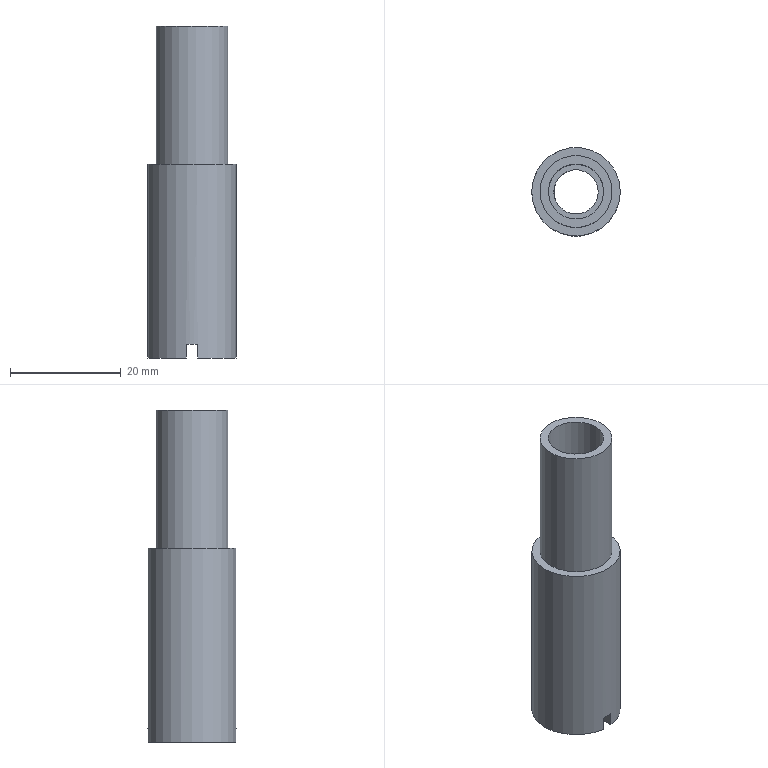Part | NX | features solid 2 | 1 solid | 15 faces | box 16 x 16 x 60 mm | volume 5886 mm3 | plane 11 | cylinder 4 | commonest cylinder face diameters 8 x1 10 x1 13 x1 16 x1
STEP:
#1=CARTESIAN_POINT('',(-774.,-102.937,70.5));
#2=VERTEX_POINT('',#1);
#3=CARTESIAN_POINT('',(-774.,-102.937,68.));
#4=VERTEX_POINT('',#3);
#5=CARTESIAN_POINT('',(-774.,-102.937,128.));
#6=DIRECTION('',(0.,0.,-1.));
#7=VECTOR('',#6,1000.);
#8=LINE('',#5,#7);
#9=EDGE_CURVE('',#2,#4,#8,.T.);
#10=ORIENTED_EDGE('',*,*,#9,.T.);
#11=CARTESIAN_POINT('',(-774.,-87.063,68.));
#12=VERTEX_POINT('',#11);
#13=CARTESIAN_POINT('',(-775.,-95.,68.));
#14=DIRECTION('',(0.,0.,1.));
#15=DIRECTION('',(1.,0.,0.));
#16=AXIS2_PLACEMENT_3D('',#13,#14,#15);
#17=CIRCLE('',#16,8.);
#18=EDGE_CURVE('',#4,#12,#17,.T.);
#19=ORIENTED_EDGE('',*,*,#18,.T.);
#20=CARTESIAN_POINT('',(-774.,-87.063,70.5));
#21=VERTEX_POINT('',#20);
#22=CARTESIAN_POINT('',(-774.,-87.063,128.));
#23=DIRECTION('',(0.,0.,-1.));
#24=VECTOR('',#23,1000.);
#25=LINE('',#22,#24);
#26=EDGE_CURVE('',#12,#21,#25,.F.);
#27=ORIENTED_EDGE('',*,*,#26,.T.);
#28=CARTESIAN_POINT('',(-776.,-87.063,70.5));
#29=VERTEX_POINT('',#28);
#30=CARTESIAN_POINT('',(-775.,-95.,70.5));
#31=DIRECTION('',(0.,0.,1.));
#32=DIRECTION('',(1.,0.,0.));
#33=AXIS2_PLACEMENT_3D('',#30,#31,#32);
#34=CIRCLE('',#33,8.);
#35=EDGE_CURVE('',#21,#29,#34,.T.);
#36=ORIENTED_EDGE('',*,*,#35,.T.);
#37=CARTESIAN_POINT('',(-776.,-87.063,68.));
#38=VERTEX_POINT('',#37);
#39=CARTESIAN_POINT('',(-776.,-87.063,128.));
#40=DIRECTION('',(0.,0.,-1.));
#41=VECTOR('',#40,1000.);
#42=LINE('',#39,#41);
#43=EDGE_CURVE('',#38,#29,#42,.F.);
#44=ORIENTED_EDGE('',*,*,#43,.F.);
#45=CARTESIAN_POINT('',(-776.,-102.937,68.));
#46=VERTEX_POINT('',#45);
#47=CARTESIAN_POINT('',(-775.,-95.,68.));
#48=DIRECTION('',(0.,0.,1.));
#49=DIRECTION('',(1.,0.,0.));
#50=AXIS2_PLACEMENT_3D('',#47,#48,#49);
#51=CIRCLE('',#50,8.);
#52=EDGE_CURVE('',#38,#46,#51,.T.);
#53=ORIENTED_EDGE('',*,*,#52,.T.);
#54=CARTESIAN_POINT('',(-776.,-102.937,70.5));
#55=VERTEX_POINT('',#54);
#56=CARTESIAN_POINT('',(-776.,-102.937,128.));
#57=DIRECTION('',(0.,0.,-1.));
#58=VECTOR('',#57,1000.);
#59=LINE('',#56,#58);
#60=EDGE_CURVE('',#55,#46,#59,.T.);
#61=ORIENTED_EDGE('',*,*,#60,.F.);
#62=CARTESIAN_POINT('',(-775.,-95.,70.5));
#63=DIRECTION('',(0.,0.,1.));
#64=DIRECTION('',(1.,0.,0.));
#65=AXIS2_PLACEMENT_3D('',#62,#63,#64);
#66=CIRCLE('',#65,8.);
#67=EDGE_CURVE('',#55,#2,#66,.T.);
#68=ORIENTED_EDGE('',*,*,#67,.T.);
#69=EDGE_LOOP('',(#10,#19,#27,#36,#44,#53,#61,#68));
#70=FACE_BOUND('',#69,.T.);
#71=CARTESIAN_POINT('',(-783.,-95.,103.));
#72=VERTEX_POINT('',#71);
#73=CARTESIAN_POINT('',(-775.,-95.,103.));
#74=DIRECTION('',(0.,0.,-1.));
#75=DIRECTION('',(-1.,0.,0.));
#76=AXIS2_PLACEMENT_3D('',#73,#74,#75);
#77=CIRCLE('',#76,8.);
#78=EDGE_CURVE('',#72,#72,#77,.F.);
#79=ORIENTED_EDGE('',*,*,#78,.F.);
#80=EDGE_LOOP('',(#79));
#81=FACE_BOUND('',#80,.T.);
#82=CARTESIAN_POINT('',(-775.,-95.,128.));
#83=DIRECTION('',(0.,0.,-1.));
#84=DIRECTION('',(1.,0.,0.));
#85=AXIS2_PLACEMENT_3D('',#82,#83,#84);
#86=CYLINDRICAL_SURFACE('',#85,8.);
#87=ADVANCED_FACE('',(#70,#81),#86,.T.);
#88=ORIENTED_EDGE('',*,*,#52,.F.);
#89=CARTESIAN_POINT('',(-776.,-91.127,68.));
#90=VERTEX_POINT('',#89);
#91=CARTESIAN_POINT('',(-776.,-87.,68.));
#92=DIRECTION('',(0.,1.,0.));
#93=VECTOR('',#92,1000.);
#94=LINE('',#91,#93);
#95=EDGE_CURVE('',#38,#90,#94,.F.);
#96=ORIENTED_EDGE('',*,*,#95,.T.);
#97=CARTESIAN_POINT('',(-776.,-98.873,68.));
#98=VERTEX_POINT('',#97);
#99=CARTESIAN_POINT('',(-775.,-95.,68.));
#100=DIRECTION('',(0.,0.,1.));
#101=DIRECTION('',(1.,0.,0.));
#102=AXIS2_PLACEMENT_3D('',#99,#100,#101);
#103=CIRCLE('',#102,4.);
#104=EDGE_CURVE('',#90,#98,#103,.T.);
#105=ORIENTED_EDGE('',*,*,#104,.T.);
#106=CARTESIAN_POINT('',(-776.,-87.,68.));
#107=DIRECTION('',(0.,1.,0.));
#108=VECTOR('',#107,1000.);
#109=LINE('',#106,#108);
#110=EDGE_CURVE('',#98,#46,#109,.F.);
#111=ORIENTED_EDGE('',*,*,#110,.T.);
#112=EDGE_LOOP('',(#88,#96,#105,#111));
#113=FACE_BOUND('',#112,.T.);
#114=CARTESIAN_POINT('',(-775.,-95.,68.));
#115=DIRECTION('',(0.,0.,-1.));
#116=DIRECTION('',(1.,0.,0.));
#117=AXIS2_PLACEMENT_3D('',#114,#115,#116);
#118=PLANE('',#117);
#119=ADVANCED_FACE('',(#113),#118,.T.);
#120=CARTESIAN_POINT('',(-774.,-98.873,68.));
#121=VERTEX_POINT('',#120);
#122=CARTESIAN_POINT('',(-774.,-87.,68.));
#123=DIRECTION('',(0.,1.,0.));
#124=VECTOR('',#123,1000.);
#125=LINE('',#122,#124);
#126=EDGE_CURVE('',#121,#4,#125,.F.);
#127=ORIENTED_EDGE('',*,*,#126,.F.);
#128=CARTESIAN_POINT('',(-774.,-91.127,68.));
#129=VERTEX_POINT('',#128);
#130=CARTESIAN_POINT('',(-775.,-95.,68.));
#131=DIRECTION('',(0.,0.,1.));
#132=DIRECTION('',(1.,0.,0.));
#133=AXIS2_PLACEMENT_3D('',#130,#131,#132);
#134=CIRCLE('',#133,4.);
#135=EDGE_CURVE('',#121,#129,#134,.T.);
#136=ORIENTED_EDGE('',*,*,#135,.T.);
#137=CARTESIAN_POINT('',(-774.,-87.,68.));
#138=DIRECTION('',(0.,1.,0.));
#139=VECTOR('',#138,1000.);
#140=LINE('',#137,#139);
#141=EDGE_CURVE('',#12,#129,#140,.F.);
#142=ORIENTED_EDGE('',*,*,#141,.F.);
#143=ORIENTED_EDGE('',*,*,#18,.F.);
#144=EDGE_LOOP('',(#127,#136,#142,#143));
#145=FACE_BOUND('',#144,.T.);
#146=CARTESIAN_POINT('',(-775.,-95.,68.));
#147=DIRECTION('',(0.,0.,-1.));
#148=DIRECTION('',(1.,0.,0.));
#149=AXIS2_PLACEMENT_3D('',#146,#147,#148);
#150=PLANE('',#149);
#151=ADVANCED_FACE('',(#145),#150,.T.);
#152=ORIENTED_EDGE('',*,*,#78,.T.);
#153=EDGE_LOOP('',(#152));
#154=FACE_BOUND('',#153,.T.);
#155=CARTESIAN_POINT('',(-768.5,-95.,103.));
#156=VERTEX_POINT('',#155);
#157=CARTESIAN_POINT('',(-775.,-95.,103.));
#158=DIRECTION('',(0.,0.,1.));
#159=DIRECTION('',(1.,0.,0.));
#160=AXIS2_PLACEMENT_3D('',#157,#158,#159);
#161=CIRCLE('',#160,6.5);
#162=EDGE_CURVE('',#156,#156,#161,.T.);
#163=ORIENTED_EDGE('',*,*,#162,.F.);
#164=EDGE_LOOP('',(#163));
#165=FACE_BOUND('',#164,.T.);
#166=CARTESIAN_POINT('',(-775.,-95.,103.));
#167=DIRECTION('',(0.,0.,1.));
#168=DIRECTION('',(-1.,0.,0.));
#169=AXIS2_PLACEMENT_3D('',#166,#167,#168);
#170=PLANE('',#169);
#171=ADVANCED_FACE('',(#154,#165),#170,.T.);
#172=CARTESIAN_POINT('',(-768.5,-95.,128.));
#173=VERTEX_POINT('',#172);
#174=CARTESIAN_POINT('',(-775.,-95.,128.));
#175=DIRECTION('',(0.,0.,1.));
#176=DIRECTION('',(1.,0.,0.));
#177=AXIS2_PLACEMENT_3D('',#174,#175,#176);
#178=CIRCLE('',#177,6.5);
#179=EDGE_CURVE('',#173,#173,#178,.T.);
#180=ORIENTED_EDGE('',*,*,#179,.F.);
#181=EDGE_LOOP('',(#180));
#182=FACE_BOUND('',#181,.T.);
#183=ORIENTED_EDGE('',*,*,#162,.T.);
#184=EDGE_LOOP('',(#183));
#185=FACE_BOUND('',#184,.T.);
#186=CARTESIAN_POINT('',(-775.,-95.,103.));
#187=DIRECTION('',(0.,0.,1.));
#188=DIRECTION('',(-1.,0.,0.));
#189=AXIS2_PLACEMENT_3D('',#186,#187,#188);
#190=CYLINDRICAL_SURFACE('',#189,6.5);
#191=ADVANCED_FACE('',(#182,#185),#190,.T.);
#192=CARTESIAN_POINT('',(-770.,-95.,128.));
#193=VERTEX_POINT('',#192);
#194=CARTESIAN_POINT('',(-775.,-95.,128.));
#195=DIRECTION('',(0.,0.,1.));
#196=DIRECTION('',(1.,0.,0.));
#197=AXIS2_PLACEMENT_3D('',#194,#195,#196);
#198=CIRCLE('',#197,5.);
#199=EDGE_CURVE('',#193,#193,#198,.T.);
#200=ORIENTED_EDGE('',*,*,#199,.F.);
#201=EDGE_LOOP('',(#200));
#202=FACE_BOUND('',#201,.T.);
#203=ORIENTED_EDGE('',*,*,#179,.T.);
#204=EDGE_LOOP('',(#203));
#205=FACE_BOUND('',#204,.T.);
#206=CARTESIAN_POINT('',(-775.,-95.,128.));
#207=DIRECTION('',(0.,0.,-1.));
#208=DIRECTION('',(1.,0.,0.));
#209=AXIS2_PLACEMENT_3D('',#206,#207,#208);
#210=PLANE('',#209);
#211=ADVANCED_FACE('',(#202,#205),#210,.F.);
#212=CARTESIAN_POINT('',(-771.,-95.,78.));
#213=VERTEX_POINT('',#212);
#214=CARTESIAN_POINT('',(-775.,-95.,78.));
#215=DIRECTION('',(0.,0.,1.));
#216=DIRECTION('',(1.,0.,0.));
#217=AXIS2_PLACEMENT_3D('',#214,#215,#216);
#218=CIRCLE('',#217,4.);
#219=EDGE_CURVE('',#213,#213,#218,.F.);
#220=ORIENTED_EDGE('',*,*,#219,.F.);
#221=EDGE_LOOP('',(#220));
#222=FACE_BOUND('',#221,.T.);
#223=ORIENTED_EDGE('',*,*,#135,.F.);
#224=CARTESIAN_POINT('',(-774.,-98.873,70.5));
#225=VERTEX_POINT('',#224);
#226=CARTESIAN_POINT('',(-774.,-98.873,78.));
#227=DIRECTION('',(0.,0.,-1.));
#228=VECTOR('',#227,1000.);
#229=LINE('',#226,#228);
#230=EDGE_CURVE('',#225,#121,#229,.T.);
#231=ORIENTED_EDGE('',*,*,#230,.F.);
#232=CARTESIAN_POINT('',(-776.,-98.873,70.5));
#233=VERTEX_POINT('',#232);
#234=CARTESIAN_POINT('',(-775.,-95.,70.5));
#235=DIRECTION('',(0.,0.,1.));
#236=DIRECTION('',(1.,0.,0.));
#237=AXIS2_PLACEMENT_3D('',#234,#235,#236);
#238=CIRCLE('',#237,4.);
#239=EDGE_CURVE('',#233,#225,#238,.T.);
#240=ORIENTED_EDGE('',*,*,#239,.F.);
#241=CARTESIAN_POINT('',(-776.,-98.873,78.));
#242=DIRECTION('',(0.,0.,-1.));
#243=VECTOR('',#242,1000.);
#244=LINE('',#241,#243);
#245=EDGE_CURVE('',#233,#98,#244,.T.);
#246=ORIENTED_EDGE('',*,*,#245,.T.);
#247=ORIENTED_EDGE('',*,*,#104,.F.);
#248=CARTESIAN_POINT('',(-776.,-91.127,70.5));
#249=VERTEX_POINT('',#248);
#250=CARTESIAN_POINT('',(-776.,-91.127,78.));
#251=DIRECTION('',(0.,0.,-1.));
#252=VECTOR('',#251,1000.);
#253=LINE('',#250,#252);
#254=EDGE_CURVE('',#90,#249,#253,.F.);
#255=ORIENTED_EDGE('',*,*,#254,.T.);
#256=CARTESIAN_POINT('',(-774.,-91.127,70.5));
#257=VERTEX_POINT('',#256);
#258=CARTESIAN_POINT('',(-775.,-95.,70.5));
#259=DIRECTION('',(0.,0.,1.));
#260=DIRECTION('',(1.,0.,0.));
#261=AXIS2_PLACEMENT_3D('',#258,#259,#260);
#262=CIRCLE('',#261,4.);
#263=EDGE_CURVE('',#257,#249,#262,.T.);
#264=ORIENTED_EDGE('',*,*,#263,.F.);
#265=CARTESIAN_POINT('',(-774.,-91.127,78.));
#266=DIRECTION('',(0.,0.,-1.));
#267=VECTOR('',#266,1000.);
#268=LINE('',#265,#267);
#269=EDGE_CURVE('',#129,#257,#268,.F.);
#270=ORIENTED_EDGE('',*,*,#269,.F.);
#271=EDGE_LOOP('',(#223,#231,#240,#246,#247,#255,#264,#270));
#272=FACE_BOUND('',#271,.T.);
#273=CARTESIAN_POINT('',(-775.,-95.,78.));
#274=DIRECTION('',(0.,0.,-1.));
#275=DIRECTION('',(1.,0.,0.));
#276=AXIS2_PLACEMENT_3D('',#273,#274,#275);
#277=CYLINDRICAL_SURFACE('',#276,4.);
#278=ADVANCED_FACE('',(#222,#272),#277,.F.);
#279=CARTESIAN_POINT('',(-770.,-95.,78.));
#280=VERTEX_POINT('',#279);
#281=CARTESIAN_POINT('',(-775.,-95.,78.));
#282=DIRECTION('',(0.,0.,1.));
#283=DIRECTION('',(1.,0.,0.));
#284=AXIS2_PLACEMENT_3D('',#281,#282,#283);
#285=CIRCLE('',#284,5.);
#286=EDGE_CURVE('',#280,#280,#285,.T.);
#287=ORIENTED_EDGE('',*,*,#286,.T.);
#288=EDGE_LOOP('',(#287));
#289=FACE_BOUND('',#288,.T.);
#290=ORIENTED_EDGE('',*,*,#219,.T.);
#291=EDGE_LOOP('',(#290));
#292=FACE_BOUND('',#291,.T.);
#293=CARTESIAN_POINT('',(-775.,-95.,78.));
#294=DIRECTION('',(0.,0.,-1.));
#295=DIRECTION('',(1.,0.,0.));
#296=AXIS2_PLACEMENT_3D('',#293,#294,#295);
#297=PLANE('',#296);
#298=ADVANCED_FACE('',(#289,#292),#297,.F.);
#299=ORIENTED_EDGE('',*,*,#199,.T.);
#300=EDGE_LOOP('',(#299));
#301=FACE_BOUND('',#300,.T.);
#302=ORIENTED_EDGE('',*,*,#286,.F.);
#303=EDGE_LOOP('',(#302));
#304=FACE_BOUND('',#303,.T.);
#305=CARTESIAN_POINT('',(-775.,-95.,128.));
#306=DIRECTION('',(0.,0.,-1.));
#307=DIRECTION('',(1.,0.,0.));
#308=AXIS2_PLACEMENT_3D('',#305,#306,#307);
#309=CYLINDRICAL_SURFACE('',#308,5.);
#310=ADVANCED_FACE('',(#301,#304),#309,.F.);
#311=ORIENTED_EDGE('',*,*,#9,.F.);
#312=CARTESIAN_POINT('',(-774.,-87.,70.5));
#313=DIRECTION('',(0.,1.,0.));
#314=VECTOR('',#313,1000.);
#315=LINE('',#312,#314);
#316=EDGE_CURVE('',#225,#2,#315,.F.);
#317=ORIENTED_EDGE('',*,*,#316,.F.);
#318=ORIENTED_EDGE('',*,*,#230,.T.);
#319=ORIENTED_EDGE('',*,*,#126,.T.);
#320=EDGE_LOOP('',(#311,#317,#318,#319));
#321=FACE_BOUND('',#320,.T.);
#322=CARTESIAN_POINT('',(-774.,-87.,68.));
#323=DIRECTION('',(1.,0.,0.));
#324=DIRECTION('',(0.,0.,1.));
#325=AXIS2_PLACEMENT_3D('',#322,#323,#324);
#326=PLANE('',#325);
#327=ADVANCED_FACE('',(#321),#326,.F.);
#328=CARTESIAN_POINT('',(-776.,-87.,70.5));
#329=DIRECTION('',(0.,1.,0.));
#330=VECTOR('',#329,1000.);
#331=LINE('',#328,#330);
#332=EDGE_CURVE('',#233,#55,#331,.F.);
#333=ORIENTED_EDGE('',*,*,#332,.T.);
#334=ORIENTED_EDGE('',*,*,#60,.T.);
#335=ORIENTED_EDGE('',*,*,#110,.F.);
#336=ORIENTED_EDGE('',*,*,#245,.F.);
#337=EDGE_LOOP('',(#333,#334,#335,#336));
#338=FACE_BOUND('',#337,.T.);
#339=CARTESIAN_POINT('',(-776.,-87.,68.));
#340=DIRECTION('',(1.,0.,0.));
#341=DIRECTION('',(0.,0.,1.));
#342=AXIS2_PLACEMENT_3D('',#339,#340,#341);
#343=PLANE('',#342);
#344=ADVANCED_FACE('',(#338),#343,.T.);
#345=ORIENTED_EDGE('',*,*,#67,.F.);
#346=ORIENTED_EDGE('',*,*,#332,.F.);
#347=ORIENTED_EDGE('',*,*,#239,.T.);
#348=ORIENTED_EDGE('',*,*,#316,.T.);
#349=EDGE_LOOP('',(#345,#346,#347,#348));
#350=FACE_BOUND('',#349,.T.);
#351=CARTESIAN_POINT('',(-775.,-87.,70.5));
#352=DIRECTION('',(0.,0.,-1.));
#353=DIRECTION('',(0.,-1.,0.));
#354=AXIS2_PLACEMENT_3D('',#351,#352,#353);
#355=PLANE('',#354);
#356=ADVANCED_FACE('',(#350),#355,.T.);
#357=ORIENTED_EDGE('',*,*,#35,.F.);
#358=CARTESIAN_POINT('',(-774.,-87.,70.5));
#359=DIRECTION('',(0.,1.,0.));
#360=VECTOR('',#359,1000.);
#361=LINE('',#358,#360);
#362=EDGE_CURVE('',#21,#257,#361,.F.);
#363=ORIENTED_EDGE('',*,*,#362,.T.);
#364=ORIENTED_EDGE('',*,*,#263,.T.);
#365=CARTESIAN_POINT('',(-776.,-87.,70.5));
#366=DIRECTION('',(0.,1.,0.));
#367=VECTOR('',#366,1000.);
#368=LINE('',#365,#367);
#369=EDGE_CURVE('',#29,#249,#368,.F.);
#370=ORIENTED_EDGE('',*,*,#369,.F.);
#371=EDGE_LOOP('',(#357,#363,#364,#370));
#372=FACE_BOUND('',#371,.T.);
#373=CARTESIAN_POINT('',(-775.,-87.,70.5));
#374=DIRECTION('',(0.,0.,-1.));
#375=DIRECTION('',(0.,-1.,0.));
#376=AXIS2_PLACEMENT_3D('',#373,#374,#375);
#377=PLANE('',#376);
#378=ADVANCED_FACE('',(#372),#377,.T.);
#379=ORIENTED_EDGE('',*,*,#26,.F.);
#380=ORIENTED_EDGE('',*,*,#141,.T.);
#381=ORIENTED_EDGE('',*,*,#269,.T.);
#382=ORIENTED_EDGE('',*,*,#362,.F.);
#383=EDGE_LOOP('',(#379,#380,#381,#382));
#384=FACE_BOUND('',#383,.T.);
#385=CARTESIAN_POINT('',(-774.,-87.,68.));
#386=DIRECTION('',(1.,0.,0.));
#387=DIRECTION('',(0.,0.,1.));
#388=AXIS2_PLACEMENT_3D('',#385,#386,#387);
#389=PLANE('',#388);
#390=ADVANCED_FACE('',(#384),#389,.F.);
#391=ORIENTED_EDGE('',*,*,#95,.F.);
#392=ORIENTED_EDGE('',*,*,#43,.T.);
#393=ORIENTED_EDGE('',*,*,#369,.T.);
#394=ORIENTED_EDGE('',*,*,#254,.F.);
#395=EDGE_LOOP('',(#391,#392,#393,#394));
#396=FACE_BOUND('',#395,.T.);
#397=CARTESIAN_POINT('',(-776.,-87.,68.));
#398=DIRECTION('',(1.,0.,0.));
#399=DIRECTION('',(0.,0.,1.));
#400=AXIS2_PLACEMENT_3D('',#397,#398,#399);
#401=PLANE('',#400);
#402=ADVANCED_FACE('',(#396),#401,.T.);
#403=CLOSED_SHELL('',(#87,#119,#151,#171,#191,#211,#278,#298,#310,#327,#344,#356,#378,#390,#402));
#404=MANIFOLD_SOLID_BREP('',#403);
#405=(LENGTH_UNIT()NAMED_UNIT(*)SI_UNIT(.MILLI.,.METRE.));
#406=UNCERTAINTY_MEASURE_WITH_UNIT(LENGTH_MEASURE(0.00001),#405,'','');
#407=(NAMED_UNIT(*)PLANE_ANGLE_UNIT()SI_UNIT($,.RADIAN.));
#408=(NAMED_UNIT(*)SI_UNIT($,.STERADIAN.)SOLID_ANGLE_UNIT());
#409=(GEOMETRIC_REPRESENTATION_CONTEXT(3)GLOBAL_UNCERTAINTY_ASSIGNED_CONTEXT((#406))GLOBAL_UNIT_ASSIGNED_CONTEXT((#405,#407,#408))REPRESENTATION_CONTEXT('',''));
#410=ADVANCED_BREP_SHAPE_REPRESENTATION('',(#404),#409);